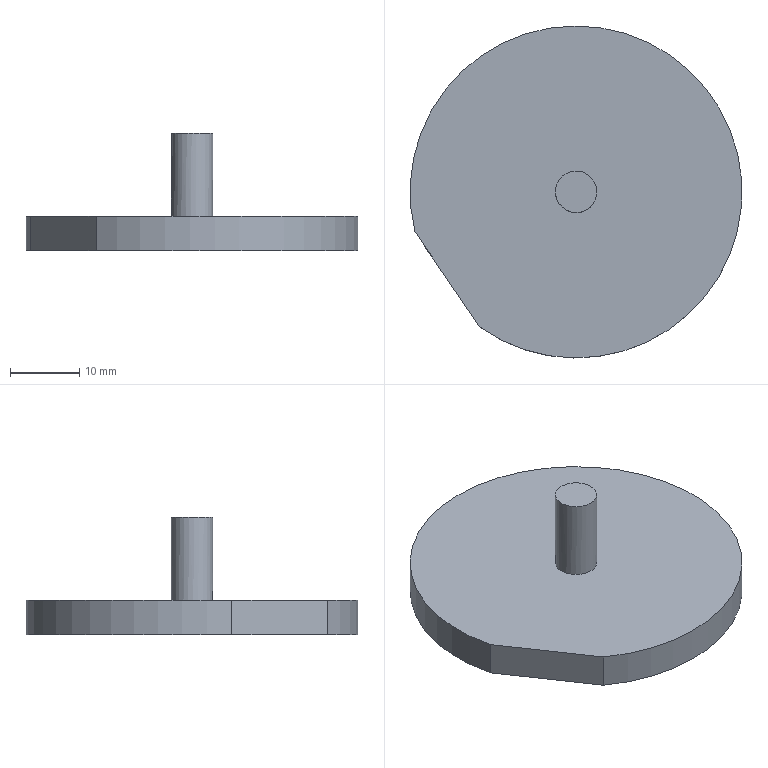Part | NX | features solid 2 | 1 solid | 6 faces | box 48 x 48 x 17 mm | volume 9303 mm3 | plane 4 | cylinder 2 | commonest cylinder face diameters 6 x1 48 x1
STEP:
#1=CARTESIAN_POINT('',(-175.382,14.71,115.));
#2=VERTEX_POINT('',#1);
#3=CARTESIAN_POINT('',(-177.504,12.589,115.));
#4=DIRECTION('',(0.,0.,1.));
#5=DIRECTION('',(0.7071,0.7071,0.));
#6=AXIS2_PLACEMENT_3D('',#3,#4,#5);
#7=CIRCLE('',#6,3.);
#8=EDGE_CURVE('',#2,#2,#7,.T.);
#9=ORIENTED_EDGE('',*,*,#8,.F.);
#10=EDGE_LOOP('',(#9));
#11=FACE_BOUND('',#10,.T.);
#12=CARTESIAN_POINT('',(-191.394,-6.983,115.));
#13=VERTEX_POINT('',#12);
#14=CARTESIAN_POINT('',(-200.8,6.82,115.));
#15=VERTEX_POINT('',#14);
#16=CARTESIAN_POINT('',(-196.097,-0.08154,115.));
#17=DIRECTION('',(-0.5631,0.8264,0.));
#18=VECTOR('',#17,1000.);
#19=LINE('',#16,#18);
#20=EDGE_CURVE('',#13,#15,#19,.T.);
#21=ORIENTED_EDGE('',*,*,#20,.F.);
#22=CARTESIAN_POINT('',(-177.504,12.589,115.));
#23=DIRECTION('',(0.,0.,-1.));
#24=DIRECTION('',(-0.8264,-0.5631,0.));
#25=AXIS2_PLACEMENT_3D('',#22,#23,#24);
#26=CIRCLE('',#25,24.);
#27=EDGE_CURVE('',#15,#13,#26,.T.);
#28=ORIENTED_EDGE('',*,*,#27,.F.);
#29=EDGE_LOOP('',(#21,#28));
#30=FACE_BOUND('',#29,.T.);
#31=CARTESIAN_POINT('',(-177.504,12.589,115.));
#32=DIRECTION('',(0.,0.,1.));
#33=DIRECTION('',(0.8264,0.5631,0.));
#34=AXIS2_PLACEMENT_3D('',#31,#32,#33);
#35=PLANE('',#34);
#36=ADVANCED_FACE('',(#11,#30),#35,.T.);
#37=CARTESIAN_POINT('',(-191.394,-6.983,110.));
#38=VERTEX_POINT('',#37);
#39=CARTESIAN_POINT('',(-200.8,6.82,110.));
#40=VERTEX_POINT('',#39);
#41=CARTESIAN_POINT('',(-211.583,22.643,110.));
#42=DIRECTION('',(-0.5631,0.8264,0.));
#43=VECTOR('',#42,1000.);
#44=LINE('',#41,#43);
#45=EDGE_CURVE('',#38,#40,#44,.T.);
#46=ORIENTED_EDGE('',*,*,#45,.T.);
#47=CARTESIAN_POINT('',(-177.504,12.589,110.));
#48=DIRECTION('',(0.,0.,1.));
#49=DIRECTION('',(0.8264,0.5631,0.));
#50=AXIS2_PLACEMENT_3D('',#47,#48,#49);
#51=CIRCLE('',#50,24.);
#52=EDGE_CURVE('',#38,#40,#51,.T.);
#53=ORIENTED_EDGE('',*,*,#52,.F.);
#54=EDGE_LOOP('',(#46,#53));
#55=FACE_BOUND('',#54,.T.);
#56=CARTESIAN_POINT('',(-177.504,12.589,110.));
#57=DIRECTION('',(0.,0.,-1.));
#58=DIRECTION('',(-0.8264,-0.5631,0.));
#59=AXIS2_PLACEMENT_3D('',#56,#57,#58);
#60=PLANE('',#59);
#61=ADVANCED_FACE('',(#55),#60,.T.);
#62=CARTESIAN_POINT('',(-200.8,6.82,110.));
#63=DIRECTION('',(0.,0.,1.));
#64=VECTOR('',#63,1000.);
#65=LINE('',#62,#64);
#66=EDGE_CURVE('',#15,#40,#65,.F.);
#67=ORIENTED_EDGE('',*,*,#66,.F.);
#68=ORIENTED_EDGE('',*,*,#27,.T.);
#69=CARTESIAN_POINT('',(-191.394,-6.983,110.));
#70=DIRECTION('',(0.,0.,1.));
#71=VECTOR('',#70,1000.);
#72=LINE('',#69,#71);
#73=EDGE_CURVE('',#38,#13,#72,.T.);
#74=ORIENTED_EDGE('',*,*,#73,.F.);
#75=ORIENTED_EDGE('',*,*,#52,.T.);
#76=EDGE_LOOP('',(#67,#68,#74,#75));
#77=FACE_BOUND('',#76,.T.);
#78=CARTESIAN_POINT('',(-177.504,12.589,110.));
#79=DIRECTION('',(0.,0.,1.));
#80=DIRECTION('',(0.8264,0.5631,0.));
#81=AXIS2_PLACEMENT_3D('',#78,#79,#80);
#82=CYLINDRICAL_SURFACE('',#81,24.);
#83=ADVANCED_FACE('',(#77),#82,.T.);
#84=ORIENTED_EDGE('',*,*,#66,.T.);
#85=ORIENTED_EDGE('',*,*,#45,.F.);
#86=ORIENTED_EDGE('',*,*,#73,.T.);
#87=ORIENTED_EDGE('',*,*,#20,.T.);
#88=EDGE_LOOP('',(#84,#85,#86,#87));
#89=FACE_BOUND('',#88,.T.);
#90=CARTESIAN_POINT('',(-211.583,22.643,110.));
#91=DIRECTION('',(0.8264,0.5631,0.));
#92=DIRECTION('',(0.,0.,-1.));
#93=AXIS2_PLACEMENT_3D('',#90,#91,#92);
#94=PLANE('',#93);
#95=ADVANCED_FACE('',(#89),#94,.F.);
#96=CARTESIAN_POINT('',(-179.983,10.9,127.));
#97=VERTEX_POINT('',#96);
#98=CARTESIAN_POINT('',(-177.504,12.589,127.));
#99=DIRECTION('',(0.,0.,-1.));
#100=DIRECTION('',(-0.8264,-0.5631,0.));
#101=AXIS2_PLACEMENT_3D('',#98,#99,#100);
#102=CIRCLE('',#101,3.);
#103=EDGE_CURVE('',#97,#97,#102,.T.);
#104=ORIENTED_EDGE('',*,*,#103,.F.);
#105=EDGE_LOOP('',(#104));
#106=FACE_BOUND('',#105,.T.);
#107=CARTESIAN_POINT('',(-177.504,12.589,127.));
#108=DIRECTION('',(0.,0.,1.));
#109=DIRECTION('',(0.8264,0.5631,0.));
#110=AXIS2_PLACEMENT_3D('',#107,#108,#109);
#111=PLANE('',#110);
#112=ADVANCED_FACE('',(#106),#111,.T.);
#113=ORIENTED_EDGE('',*,*,#103,.T.);
#114=EDGE_LOOP('',(#113));
#115=FACE_BOUND('',#114,.T.);
#116=ORIENTED_EDGE('',*,*,#8,.T.);
#117=EDGE_LOOP('',(#116));
#118=FACE_BOUND('',#117,.T.);
#119=CARTESIAN_POINT('',(-177.504,12.589,115.));
#120=DIRECTION('',(0.,0.,1.));
#121=DIRECTION('',(0.8264,0.5631,0.));
#122=AXIS2_PLACEMENT_3D('',#119,#120,#121);
#123=CYLINDRICAL_SURFACE('',#122,3.);
#124=ADVANCED_FACE('',(#115,#118),#123,.T.);
#125=CLOSED_SHELL('',(#36,#61,#83,#95,#112,#124));
#126=MANIFOLD_SOLID_BREP('',#125);
#127=(LENGTH_UNIT()NAMED_UNIT(*)SI_UNIT(.MILLI.,.METRE.));
#128=UNCERTAINTY_MEASURE_WITH_UNIT(LENGTH_MEASURE(0.00001),#127,'','');
#129=(NAMED_UNIT(*)PLANE_ANGLE_UNIT()SI_UNIT($,.RADIAN.));
#130=(NAMED_UNIT(*)SI_UNIT($,.STERADIAN.)SOLID_ANGLE_UNIT());
#131=(GEOMETRIC_REPRESENTATION_CONTEXT(3)GLOBAL_UNCERTAINTY_ASSIGNED_CONTEXT((#128))GLOBAL_UNIT_ASSIGNED_CONTEXT((#127,#129,#130))REPRESENTATION_CONTEXT('',''));
#132=ADVANCED_BREP_SHAPE_REPRESENTATION('',(#126),#131);